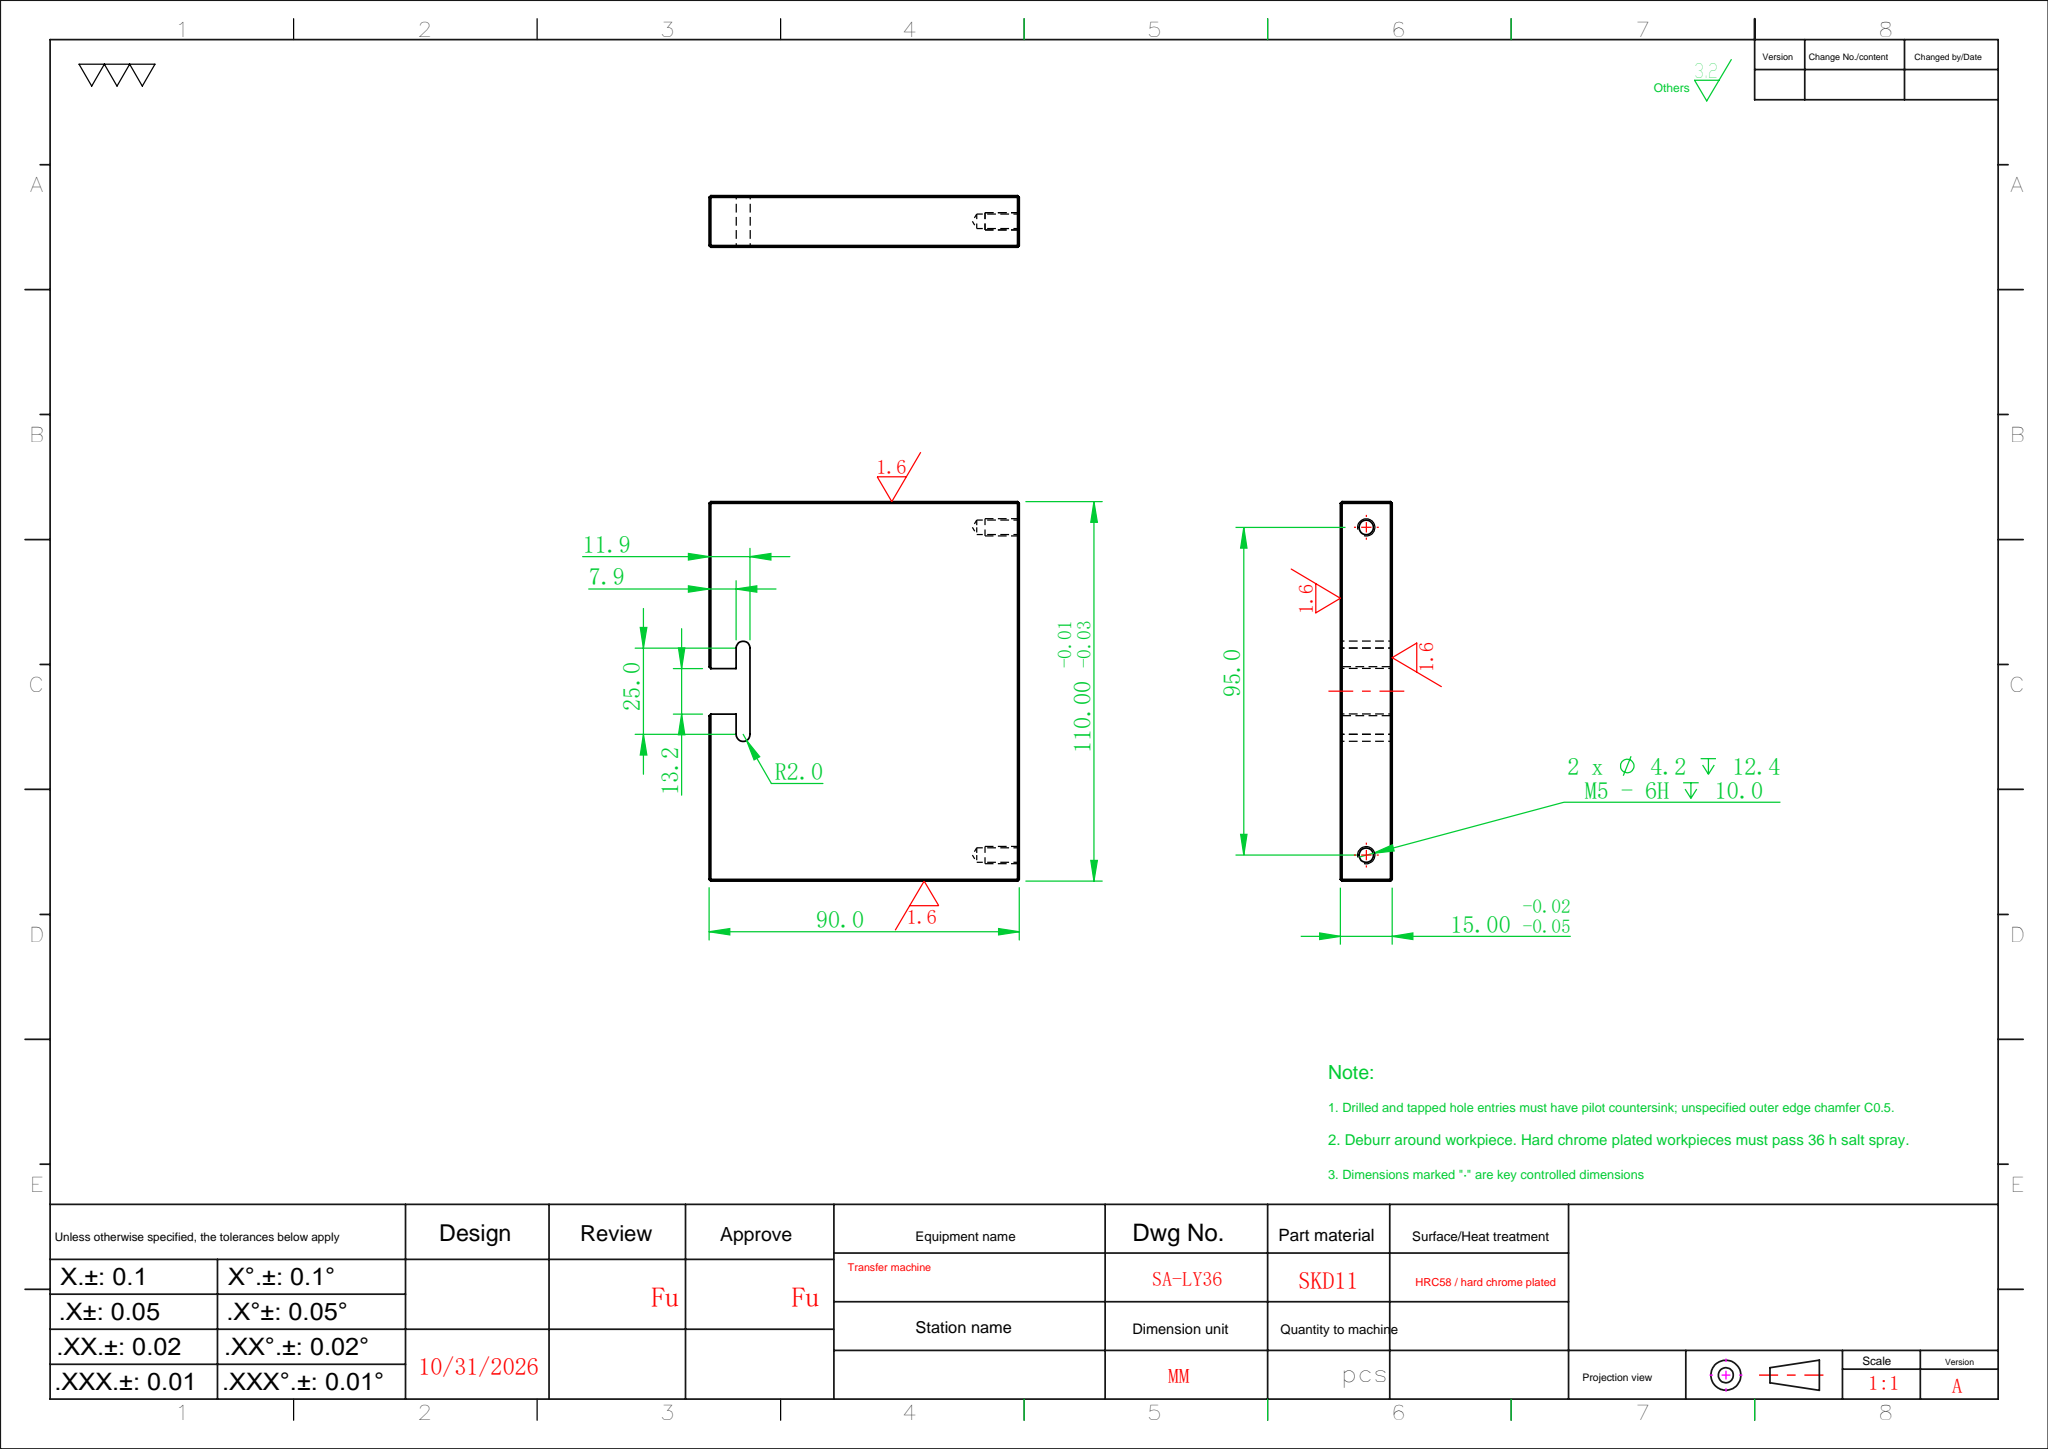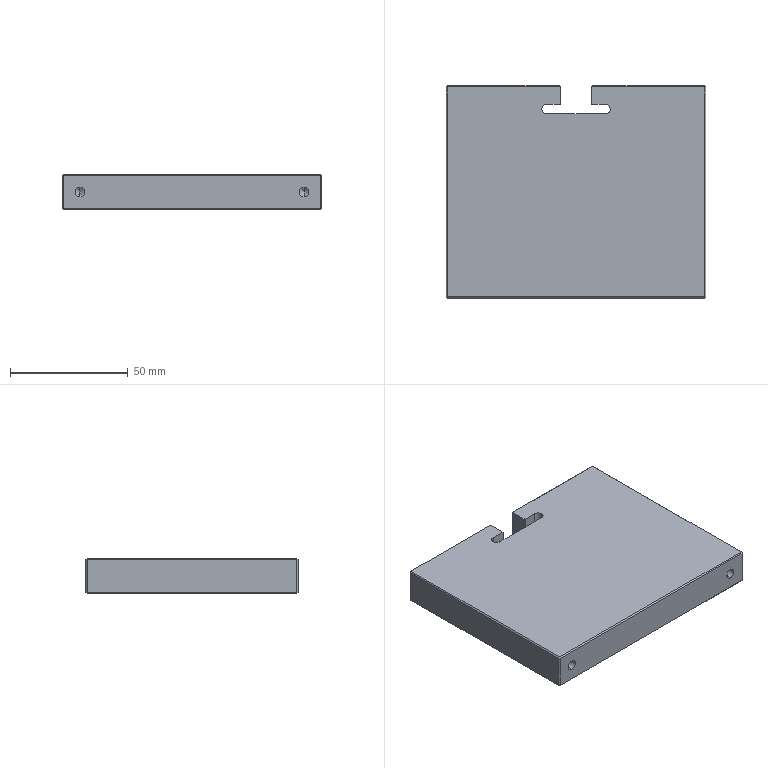Part | SolidWorks | features Cut 2, Chamfer 1, Extrusion 1, HoleWzd 1 | 1 solid | 47 faces | box 110 x 90 x 15 mm | volume 144771 mm3 | plane 36 | cylinder 7 | cone 4 | commonest cylinder face diameters 4.2 x4 4.05 x3